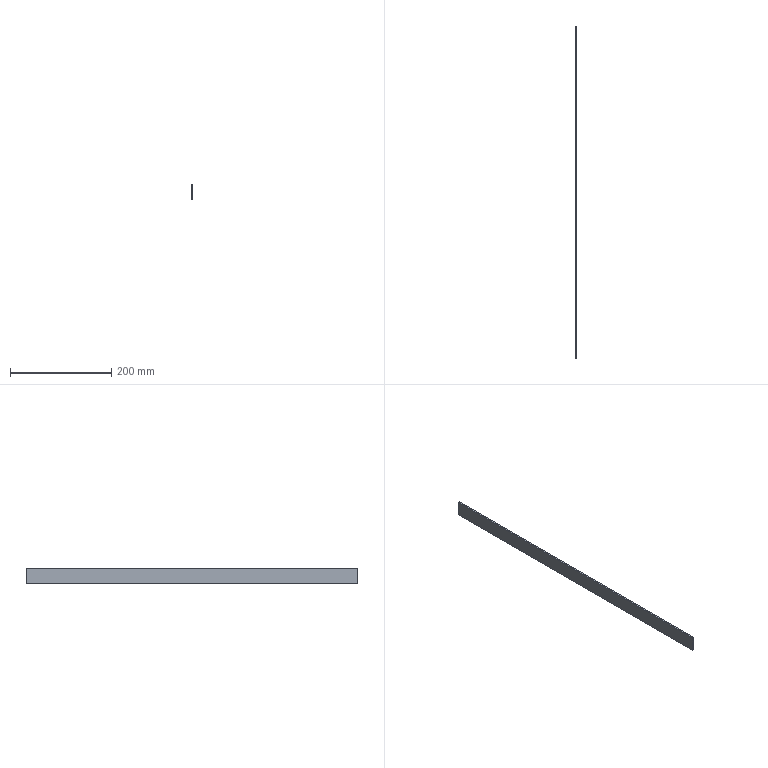Part | SolidWorks | 1 solid | 6 faces | box 3 x 656 x 30 mm | volume 59040 mm3 | plane 6
STEP:
#1=CARTESIAN_POINT('',(0.,328.,15.));
#2=VERTEX_POINT('',#1);
#3=CARTESIAN_POINT('',(0.,-328.,15.));
#4=VERTEX_POINT('',#3);
#5=CARTESIAN_POINT('',(0.,-328.,15.));
#6=DIRECTION('',(0.,-1.,0.));
#7=VECTOR('',#6,1000.);
#8=LINE('',#5,#7);
#9=EDGE_CURVE('',#2,#4,#8,.T.);
#10=ORIENTED_EDGE('',*,*,#9,.F.);
#11=CARTESIAN_POINT('',(-3.,328.,15.));
#12=VERTEX_POINT('',#11);
#13=CARTESIAN_POINT('',(-3.,328.,15.));
#14=DIRECTION('',(1.,0.,0.));
#15=VECTOR('',#14,1000.);
#16=LINE('',#13,#15);
#17=EDGE_CURVE('',#12,#2,#16,.T.);
#18=ORIENTED_EDGE('',*,*,#17,.F.);
#19=CARTESIAN_POINT('',(-3.,-328.,15.));
#20=VERTEX_POINT('',#19);
#21=CARTESIAN_POINT('',(-3.,-328.,15.));
#22=DIRECTION('',(0.,-1.,0.));
#23=VECTOR('',#22,1000.);
#24=LINE('',#21,#23);
#25=EDGE_CURVE('',#12,#20,#24,.T.);
#26=ORIENTED_EDGE('',*,*,#25,.T.);
#27=CARTESIAN_POINT('',(-3.,-328.,15.));
#28=DIRECTION('',(1.,0.,0.));
#29=VECTOR('',#28,1000.);
#30=LINE('',#27,#29);
#31=EDGE_CURVE('',#20,#4,#30,.T.);
#32=ORIENTED_EDGE('',*,*,#31,.T.);
#33=EDGE_LOOP('',(#10,#18,#26,#32));
#34=FACE_OUTER_BOUND('',#33,.T.);
#35=CARTESIAN_POINT('',(-3.,-328.,15.));
#36=DIRECTION('',(0.,0.,1.));
#37=DIRECTION('',(1.,0.,0.));
#38=AXIS2_PLACEMENT_3D('',#35,#36,#37);
#39=PLANE('',#38);
#40=ADVANCED_FACE('',(#34),#39,.T.);
#41=CARTESIAN_POINT('',(0.,328.,-15.));
#42=VERTEX_POINT('',#41);
#43=CARTESIAN_POINT('',(0.,328.,-15.));
#44=DIRECTION('',(0.,0.,1.));
#45=VECTOR('',#44,1000.);
#46=LINE('',#43,#45);
#47=EDGE_CURVE('',#42,#2,#46,.T.);
#48=ORIENTED_EDGE('',*,*,#47,.F.);
#49=CARTESIAN_POINT('',(-3.,328.,-15.));
#50=VERTEX_POINT('',#49);
#51=CARTESIAN_POINT('',(-3.,328.,-15.));
#52=DIRECTION('',(1.,0.,0.));
#53=VECTOR('',#52,1000.);
#54=LINE('',#51,#53);
#55=EDGE_CURVE('',#50,#42,#54,.T.);
#56=ORIENTED_EDGE('',*,*,#55,.F.);
#57=CARTESIAN_POINT('',(-3.,328.,-15.));
#58=DIRECTION('',(0.,0.,1.));
#59=VECTOR('',#58,1000.);
#60=LINE('',#57,#59);
#61=EDGE_CURVE('',#50,#12,#60,.T.);
#62=ORIENTED_EDGE('',*,*,#61,.T.);
#63=ORIENTED_EDGE('',*,*,#17,.T.);
#64=EDGE_LOOP('',(#48,#56,#62,#63));
#65=FACE_OUTER_BOUND('',#64,.T.);
#66=CARTESIAN_POINT('',(-3.,328.,-15.));
#67=DIRECTION('',(0.,1.,0.));
#68=DIRECTION('',(0.,0.,1.));
#69=AXIS2_PLACEMENT_3D('',#66,#67,#68);
#70=PLANE('',#69);
#71=ADVANCED_FACE('',(#65),#70,.T.);
#72=CARTESIAN_POINT('',(0.,-328.,-15.));
#73=VERTEX_POINT('',#72);
#74=CARTESIAN_POINT('',(0.,-328.,-15.));
#75=DIRECTION('',(0.,1.,0.));
#76=VECTOR('',#75,1000.);
#77=LINE('',#74,#76);
#78=EDGE_CURVE('',#73,#42,#77,.T.);
#79=ORIENTED_EDGE('',*,*,#78,.F.);
#80=CARTESIAN_POINT('',(-3.,-328.,-15.));
#81=VERTEX_POINT('',#80);
#82=CARTESIAN_POINT('',(-3.,-328.,-15.));
#83=DIRECTION('',(1.,0.,0.));
#84=VECTOR('',#83,1000.);
#85=LINE('',#82,#84);
#86=EDGE_CURVE('',#81,#73,#85,.T.);
#87=ORIENTED_EDGE('',*,*,#86,.F.);
#88=CARTESIAN_POINT('',(-3.,-328.,-15.));
#89=DIRECTION('',(0.,1.,0.));
#90=VECTOR('',#89,1000.);
#91=LINE('',#88,#90);
#92=EDGE_CURVE('',#81,#50,#91,.T.);
#93=ORIENTED_EDGE('',*,*,#92,.T.);
#94=ORIENTED_EDGE('',*,*,#55,.T.);
#95=EDGE_LOOP('',(#79,#87,#93,#94));
#96=FACE_OUTER_BOUND('',#95,.T.);
#97=CARTESIAN_POINT('',(-3.,-328.,-15.));
#98=DIRECTION('',(0.,0.,-1.));
#99=DIRECTION('',(-1.,0.,0.));
#100=AXIS2_PLACEMENT_3D('',#97,#98,#99);
#101=PLANE('',#100);
#102=ADVANCED_FACE('',(#96),#101,.T.);
#103=CARTESIAN_POINT('',(0.,-328.,-15.));
#104=DIRECTION('',(0.,0.,-1.));
#105=VECTOR('',#104,1000.);
#106=LINE('',#103,#105);
#107=EDGE_CURVE('',#4,#73,#106,.T.);
#108=ORIENTED_EDGE('',*,*,#107,.F.);
#109=ORIENTED_EDGE('',*,*,#31,.F.);
#110=CARTESIAN_POINT('',(-3.,-328.,-15.));
#111=DIRECTION('',(0.,0.,-1.));
#112=VECTOR('',#111,1000.);
#113=LINE('',#110,#112);
#114=EDGE_CURVE('',#20,#81,#113,.T.);
#115=ORIENTED_EDGE('',*,*,#114,.T.);
#116=ORIENTED_EDGE('',*,*,#86,.T.);
#117=EDGE_LOOP('',(#108,#109,#115,#116));
#118=FACE_OUTER_BOUND('',#117,.T.);
#119=CARTESIAN_POINT('',(-3.,-328.,-15.));
#120=DIRECTION('',(0.,-1.,0.));
#121=DIRECTION('',(0.,0.,-1.));
#122=AXIS2_PLACEMENT_3D('',#119,#120,#121);
#123=PLANE('',#122);
#124=ADVANCED_FACE('',(#118),#123,.T.);
#125=ORIENTED_EDGE('',*,*,#25,.F.);
#126=ORIENTED_EDGE('',*,*,#61,.F.);
#127=ORIENTED_EDGE('',*,*,#92,.F.);
#128=ORIENTED_EDGE('',*,*,#114,.F.);
#129=EDGE_LOOP('',(#125,#126,#127,#128));
#130=FACE_OUTER_BOUND('',#129,.T.);
#131=CARTESIAN_POINT('',(-3.,0.,0.));
#132=DIRECTION('',(1.,0.,0.));
#133=DIRECTION('',(0.,0.,-1.));
#134=AXIS2_PLACEMENT_3D('',#131,#132,#133);
#135=PLANE('',#134);
#136=ADVANCED_FACE('',(#130),#135,.F.);
#137=ORIENTED_EDGE('',*,*,#9,.T.);
#138=ORIENTED_EDGE('',*,*,#107,.T.);
#139=ORIENTED_EDGE('',*,*,#78,.T.);
#140=ORIENTED_EDGE('',*,*,#47,.T.);
#141=EDGE_LOOP('',(#137,#138,#139,#140));
#142=FACE_OUTER_BOUND('',#141,.T.);
#143=CARTESIAN_POINT('',(0.,0.,0.));
#144=DIRECTION('',(1.,0.,0.));
#145=DIRECTION('',(0.,0.,-1.));
#146=AXIS2_PLACEMENT_3D('',#143,#144,#145);
#147=PLANE('',#146);
#148=ADVANCED_FACE('',(#142),#147,.T.);
#149=CLOSED_SHELL('',(#40,#71,#102,#124,#136,#148));
#150=MANIFOLD_SOLID_BREP('',#149);
#151=CARTESIAN_POINT('',(0.,0.,0.));
#152=DIRECTION('',(0.,0.,1.));
#153=DIRECTION('',(1.,0.,0.));
#154=AXIS2_PLACEMENT_3D('',#151,#152,#153);
#155=(LENGTH_UNIT()NAMED_UNIT(*)SI_UNIT(.MILLI.,.METRE.));
#156=UNCERTAINTY_MEASURE_WITH_UNIT(LENGTH_MEASURE(0.00001),#155,'','');
#157=(NAMED_UNIT(*)PLANE_ANGLE_UNIT()SI_UNIT($,.RADIAN.));
#158=(NAMED_UNIT(*)SI_UNIT($,.STERADIAN.)SOLID_ANGLE_UNIT());
#159=(GEOMETRIC_REPRESENTATION_CONTEXT(3)GLOBAL_UNCERTAINTY_ASSIGNED_CONTEXT((#156))GLOBAL_UNIT_ASSIGNED_CONTEXT((#155,#157,#158))REPRESENTATION_CONTEXT('',''));
#160=ADVANCED_BREP_SHAPE_REPRESENTATION('',(#150,#154),#159);